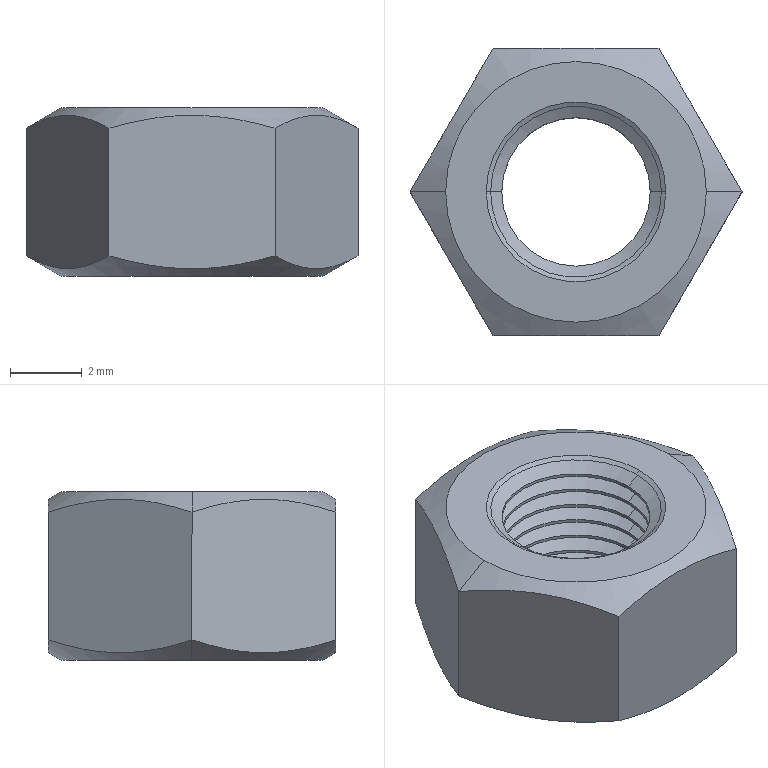Part | STEP file | hex nuts, style 1-grades ab gb_GB_FASTENER_NUT_SNAB1 M5-S | 1 solid | 68 faces | box 9.238 x 8 x 4.7 mm | volume 181.423 mm3 | cone 44 | cylinder 16 | plane 8 | commonest cylinder face diameters 4.134 x16